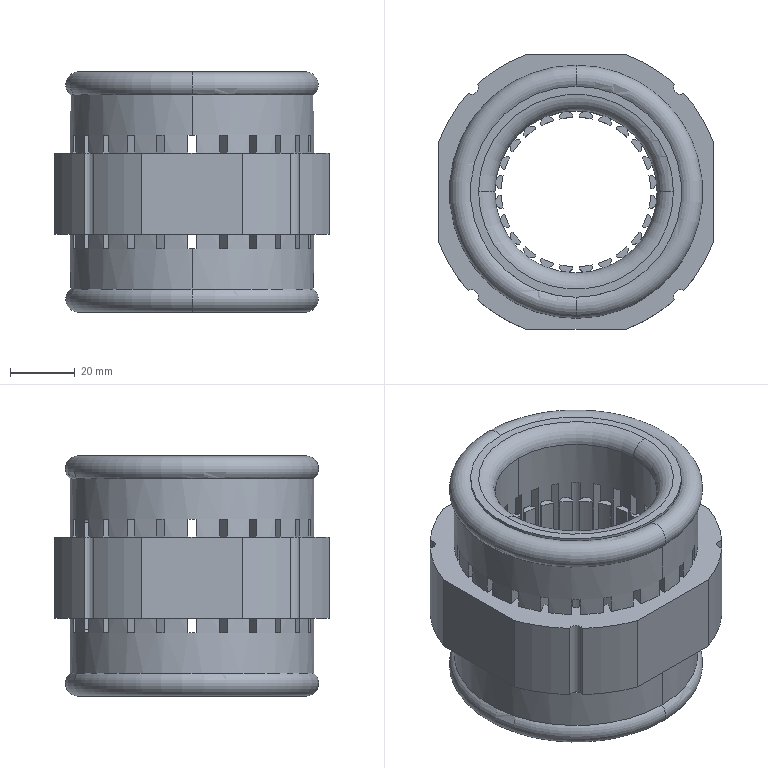Part | STEP file | MSBR-5_1_1_1_1 | 1 solid | 381 faces | box 84.5 x 84.5 x 74 mm | volume 208424 mm3 | plane 296 | cylinder 77 | torus 8 | commonest cylinder face diameters 5.6 x27 46 x24 90 x8 4.2 x6 64.98 x4 75 x4